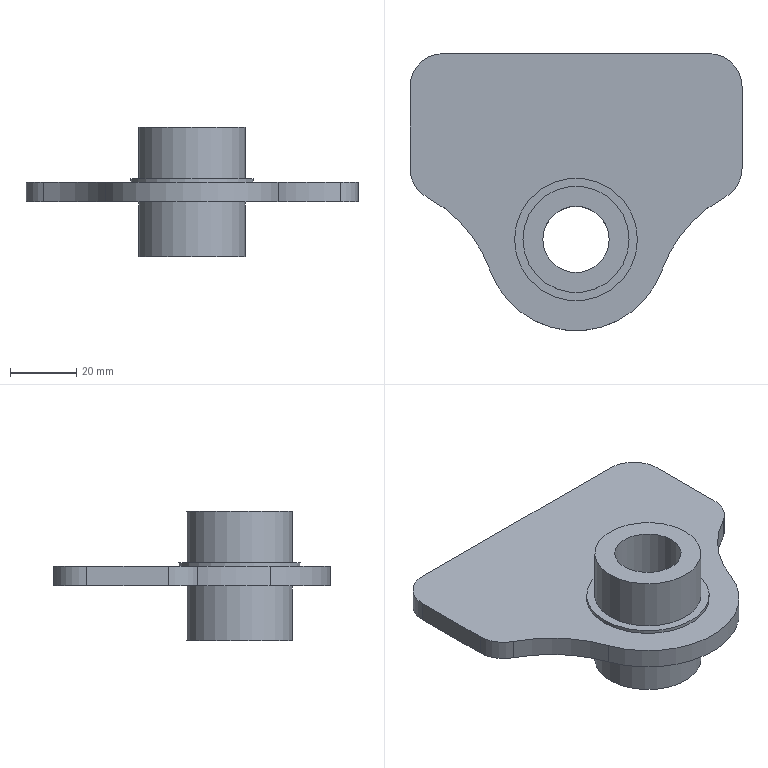NC program | NX | posted with a generic post | part box 100 x 83.5 x 39 mm
Lines 1 to 906 of 3591:
N10 G17 G21 G94 G90
(ADAPTIVE_MILLING , TOOL : D16-48-D16-100-3T-FINISH)
N12 T01 M6
N14 G53
N16 G17 G0 G90 X-29.129 Y-11.877 S3000 M3
N18 G43 Z30. H1
N20 Z3.15
N22 G94 G1 X-28.979 Y-11.865 Z2.213 F2000.
N24 X-28.829 Y-11.854 Z1.842
N26 X-28.68 Y-11.842 Z1.57
N28 X-28.53 Y-11.831 Z1.35
N30 X-28.381 Y-11.819 Z1.166
N32 X-28.231 Y-11.808 Z1.008
N34 X-28.082 Y-11.796 Z0.87
N36 X-27.932 Y-11.785 Z0.75
N38 X-27.783 Y-11.773 Z0.645
N40 X-27.633 Y-11.762 Z0.552
N42 X-27.483 Y-11.75 Z0.471
N44 X-27.334 Y-11.739 Z0.4
N46 X-27.184 Y-11.727 Z0.34
N48 X-27.035 Y-11.716 Z0.288
N50 X-26.885 Y-11.704 Z0.245
N52 X-26.736 Y-11.693 Z0.211
N54 X-26.586 Y-11.681 Z0.184
N56 X-26.436 Y-11.67 Z0.165
N58 X-26.287 Y-11.658 Z0.154
N60 X-26.137 Y-11.647 Z0.15
N62 X-24.02 Y-11.484
N64 G3 X-22.555 Y-9.578 R1.616
N66 G1 X-23.473 Y-5.647
N68 G2 X-22.056 Y9.568 R25.074
N70 X-20.662 Y-12.268 R-24.039
N72 X-23.288 Y-4.358 R24.506
N74 X-17.653 Y15.653 R24.1
N76 X-19.314 Y-13.525 R-23.593
N78 X-23.013 Y-3.231 R23.544
N80 X-13.785 Y18.59 R23.495
N82 X-17.92 Y-14.622 R-23.141
N84 X-22.633 Y-2.662 R22.849
N86 X-11.014 Y19.837 R22.99
N88 X-16.545 Y-15.504 R-22.686
N90 X-22.228 Y-2.182 R22.315
N92 X-8.532 Y20.527 R22.498
N94 X-15.335 Y-16.071 R-22.227
N96 X-21.826 Y-1.358 R21.88
N98 X-5.19 Y21.138 R21.988
N100 X-14.251 Y-16.427 R-21.762
N102 X-21.39 Y-0.363 R21.453
N104 X-1.126 Y21.266 R21.473
N106 X-12.994 Y-16.848 R-21.29
N108 X-20.917 Y0.217 R20.985
N110 X1.005 Y20.795 R20.982
N112 X-12.004 Y-16.984 R-20.813
N114 X-20.383 Y1.367 R20.542
N116 X4.974 Y19.719 R20.469
N118 X-11.011 Y-17.069 R-20.328
N120 X-19.791 Y2.388 R20.075
N122 X7.915 Y18.2 R19.96
N124 X-10.001 Y-17.112 R-19.835
N126 X-19.13 Y3.418 R19.594
N128 X10.367 Y16.335 R19.447
N130 X-9.145 Y-17.018 R19.333
N132 X-18.337 Y4.66 R19.106
N134 X12.992 Y13.643 R18.923
N136 X-8.398 Y-16.83 R18.82
N138 X-16.984 Y7.044 R18.615
N140 X17.291 Y6.061 R18.375
N142 X-8.2 Y-16.341 R18.285
N144 X-13.274 Y11.907 R18.121
N146 X-17.828 Y-0.094 R-17.828
N148 G1 X-17.825 Y0.056 Z0.154
N150 X-17.823 Y0.206 Z0.165
N152 X-17.821 Y0.356 Z0.184
N154 X-17.818 Y0.506 Z0.211
N156 X-17.816 Y0.656 Z0.245
N158 X-17.813 Y0.806 Z0.288
N160 X-17.811 Y0.956 Z0.34
N162 X-17.809 Y1.106 Z0.4
N164 X-17.806 Y1.256 Z0.471
N166 X-17.804 Y1.406 Z0.552
N168 X-17.802 Y1.556 Z0.645
N170 X-17.799 Y1.706 Z0.75
N172 X-17.797 Y1.856 Z0.87
N174 X-17.795 Y2.006 Z1.008
N176 X-17.792 Y2.156 Z1.166
N178 X-17.79 Y2.306 Z1.35
N180 X-17.788 Y2.456 Z1.57
N182 X-17.785 Y2.606 Z1.842
N184 X-17.783 Y2.756 Z2.213
N186 X-17.78 Y2.906 Z3.15
N188 G0 Z30.
(PLANAR_MILL_1_COPY , TOOL : D16-48-D16-100-3T-FINISH)
N190 X-13.655 Y22.716
N192 Z-12.4
N194 G1 X-12.158 Y23.58 Z-12.409 F1000.
N196 X-8.916 Y24.987 Z-12.428
N198 X-5.517 Y25.95 Z-12.446
N200 X-2.019 Y26.453 Z-12.465
N202 X1.514 Y26.487 Z-12.483
N204 X5.02 Y26.051 Z-12.502
N206 X8.438 Y25.152 Z-12.52
N208 X11.706 Y23.808 Z-12.539
N210 X14.766 Y22.041 Z-12.557
N212 X17.564 Y19.884 Z-12.576
N214 X20.05 Y17.373 Z-12.594
N216 X22.181 Y14.555 Z-12.613
N218 X23.919 Y11.478 Z-12.631
N220 X25.232 Y8.197 Z-12.65
N222 X26.097 Y4.772 Z-12.668
N224 X26.5 Y1.261 Z-12.687
N226 Y-1.261 Z-12.7
N228 X26.093 Y-4.794 Z-12.718
N230 X25.218 Y-8.241 Z-12.737
N232 X23.889 Y-11.54 Z-12.756
N234 X22.131 Y-14.631 Z-12.774
N236 X19.975 Y-17.46 Z-12.793
N238 X17.46 Y-19.975 Z-12.812
N240 X14.631 Y-22.131 Z-12.83
N242 X11.54 Y-23.889 Z-12.849
N244 X8.241 Y-25.218 Z-12.867
N246 X4.794 Y-26.093 Z-12.886
N248 X1.261 Y-26.5 Z-12.905
N250 X-1.261 Z-12.918
N252 X-4.087 Y-26.213 Z-12.933
N254 X-6.866 Y-25.626 Z-12.948
N256 X-9.567 Y-24.745 Z-12.962
N258 X-12.158 Y-23.58 Z-12.977
N260 X-14.342 Y-22.319 Z-12.991
N262 X-17.181 Y-20.215 Z-13.009
N264 X-19.715 Y-17.753 Z-13.028
N266 X-21.899 Y-14.975 Z-13.046
N268 X-23.695 Y-11.932 Z-13.065
N270 X-25.071 Y-8.677 Z-13.083
N272 X-26.002 Y-5.269 Z-13.102
N274 X-26.471 Y-1.767 Z-13.12
N276 Y1.767 Z-13.139
N278 X-26.002 Y5.269 Z-13.157
N280 X-25.071 Y8.677 Z-13.176
N282 X-23.695 Y11.932 Z-13.194
N284 X-21.899 Y14.975 Z-13.213
N286 X-19.715 Y17.753 Z-13.231
N288 X-17.181 Y20.215 Z-13.25
N290 X-14.342 Y22.319 Z-13.268
N292 X-12.158 Y23.58 Z-13.281
N294 X-8.916 Y24.987 Z-13.3
N296 X-5.517 Y25.95 Z-13.318
N298 X-2.019 Y26.453 Z-13.337
N300 X1.514 Y26.487 Z-13.355
N302 X5.02 Y26.051 Z-13.374
N304 X8.438 Y25.152 Z-13.392
N306 X11.706 Y23.808 Z-13.411
N308 X14.766 Y22.041 Z-13.429
N310 X17.564 Y19.884 Z-13.448
N312 X20.05 Y17.373 Z-13.466
N314 X22.181 Y14.555 Z-13.485
N316 X23.919 Y11.478 Z-13.503
N318 X25.232 Y8.197 Z-13.522
N320 X26.097 Y4.772 Z-13.54
N322 X26.5 Y1.261 Z-13.559
N324 Y-1.261 Z-13.572
N326 X26.093 Y-4.794 Z-13.591
N328 X25.218 Y-8.241 Z-13.609
N330 X23.889 Y-11.54 Z-13.628
N332 X22.131 Y-14.631 Z-13.646
N334 X19.975 Y-17.46 Z-13.665
N336 X17.46 Y-19.975 Z-13.684
N338 X14.631 Y-22.131 Z-13.702
N340 X11.54 Y-23.889 Z-13.721
N342 X8.241 Y-25.218 Z-13.74
N344 X4.794 Y-26.093 Z-13.758
N346 X1.261 Y-26.5 Z-13.777
N348 X-1.261 Z-13.79
N350 X-4.087 Y-26.213 Z-13.805
N352 X-6.866 Y-25.626 Z-13.82
N354 X-9.567 Y-24.745 Z-13.835
N356 X-12.158 Y-23.58 Z-13.85
N358 X-14.342 Y-22.319 Z-13.863
N360 X-17.181 Y-20.215 Z-13.881
N362 X-19.715 Y-17.753 Z-13.9
N364 X-21.899 Y-14.975 Z-13.918
N366 X-23.695 Y-11.932 Z-13.937
N368 X-25.071 Y-8.677 Z-13.955
N370 X-26.002 Y-5.269 Z-13.974
N372 X-26.471 Y-1.767 Z-13.992
N374 Y1.767 Z-14.011
N376 X-26.002 Y5.269 Z-14.029
N378 X-25.071 Y8.677 Z-14.048
N380 X-23.695 Y11.932 Z-14.066
N382 X-21.899 Y14.975 Z-14.085
N384 X-19.715 Y17.753 Z-14.103
N386 X-17.181 Y20.215 Z-14.122
N388 X-14.342 Y22.319 Z-14.14
N390 X-12.158 Y23.58 Z-14.153
N392 X-8.916 Y24.987 Z-14.172
N394 X-5.517 Y25.95 Z-14.19
N396 X-2.019 Y26.453 Z-14.209
N398 X1.514 Y26.487 Z-14.227
N400 X5.02 Y26.051 Z-14.246
N402 X8.438 Y25.152 Z-14.264
N404 X11.706 Y23.808 Z-14.283
N406 X14.766 Y22.041 Z-14.301
N408 X17.564 Y19.884 Z-14.32
N410 X20.05 Y17.373 Z-14.338
N412 X22.181 Y14.555 Z-14.357
N414 X23.919 Y11.478 Z-14.375
N416 X25.232 Y8.197 Z-14.394
N418 X26.097 Y4.772 Z-14.412
N420 X26.5 Y1.261 Z-14.431
N422 Y-1.261 Z-14.444
N424 X26.093 Y-4.794 Z-14.463
N426 X25.218 Y-8.241 Z-14.481
N428 X23.889 Y-11.54 Z-14.5
N430 X22.131 Y-14.631 Z-14.519
N432 X19.975 Y-17.46 Z-14.537
N434 X17.46 Y-19.975 Z-14.556
N436 X14.631 Y-22.131 Z-14.575
N438 X11.54 Y-23.889 Z-14.593
N440 X8.241 Y-25.218 Z-14.612
N442 X4.794 Y-26.093 Z-14.63
N444 X1.261 Y-26.5 Z-14.649
N446 X-1.261 Z-14.662
N448 X-4.087 Y-26.213 Z-14.677
N450 X-6.866 Y-25.626 Z-14.692
N452 X-9.567 Y-24.745 Z-14.707
N454 X-12.158 Y-23.58 Z-14.722
N456 X-14.342 Y-22.319 Z-14.735
N458 X-17.181 Y-20.215 Z-14.753
N460 X-19.715 Y-17.753 Z-14.772
N462 X-21.899 Y-14.975 Z-14.79
N464 X-23.695 Y-11.932 Z-14.809
N466 X-25.071 Y-8.677 Z-14.827
N468 X-26.002 Y-5.269 Z-14.846
N470 X-26.471 Y-1.767 Z-14.864
N472 Y1.767 Z-14.883
N474 X-26.002 Y5.269 Z-14.901
N476 X-25.071 Y8.677 Z-14.92
N478 X-23.695 Y11.932 Z-14.938
N480 X-21.899 Y14.975 Z-14.957
N482 X-19.715 Y17.753 Z-14.975
N484 X-17.181 Y20.215 Z-14.994
N486 X-14.342 Y22.319 Z-15.012
N488 X-12.158 Y23.58 Z-15.026
N490 X-8.916 Y24.987 Z-15.044
N492 X-5.517 Y25.95 Z-15.063
N494 X-2.019 Y26.453 Z-15.081
N496 X1.514 Y26.487 Z-15.1
N498 X5.02 Y26.051 Z-15.118
N500 X8.438 Y25.152 Z-15.137
N502 X11.706 Y23.808 Z-15.155
N504 X14.766 Y22.041 Z-15.174
N506 X17.564 Y19.884 Z-15.192
N508 X20.05 Y17.373 Z-15.211
N510 X22.181 Y14.555 Z-15.229
N512 X23.919 Y11.478 Z-15.248
N514 X25.232 Y8.197 Z-15.266
N516 X26.097 Y4.772 Z-15.285
N518 X26.5 Y1.261 Z-15.303
N520 Y-1.261 Z-15.316
N522 X26.093 Y-4.794 Z-15.335
N524 X25.218 Y-8.241 Z-15.354
N526 X23.889 Y-11.54 Z-15.372
N528 X22.131 Y-14.631 Z-15.391
N530 X19.975 Y-17.46 Z-15.409
N532 X17.46 Y-19.975 Z-15.428
N534 X14.631 Y-22.131 Z-15.447
N536 X11.54 Y-23.889 Z-15.465
N538 X8.241 Y-25.218 Z-15.484
N540 X4.794 Y-26.093 Z-15.503
N542 X1.261 Y-26.5 Z-15.521
N544 X-1.261 Z-15.534
N546 X-4.087 Y-26.213 Z-15.549
N548 X-6.866 Y-25.626 Z-15.564
N550 X-9.567 Y-24.745 Z-15.579
N552 X-12.158 Y-23.58 Z-15.594
N554 X-14.342 Y-22.319 Z-15.607
N556 X-17.181 Y-20.215 Z-15.626
N558 X-19.715 Y-17.753 Z-15.644
N560 X-21.899 Y-14.975 Z-15.663
N562 X-23.695 Y-11.932 Z-15.681
N564 X-25.071 Y-8.677 Z-15.7
N566 X-26.002 Y-5.269 Z-15.718
N568 X-26.471 Y-1.767 Z-15.737
N570 Y1.767 Z-15.755
N572 X-26.002 Y5.269 Z-15.774
N574 X-25.071 Y8.677 Z-15.792
N576 X-23.695 Y11.932 Z-15.811
N578 X-21.899 Y14.975 Z-15.829
N580 X-19.715 Y17.753 Z-15.848
N582 X-17.181 Y20.215 Z-15.866
N584 X-14.342 Y22.319 Z-15.885
N586 X-12.158 Y23.58 Z-15.898
N588 X-8.916 Y24.987 Z-15.916
N590 X-5.517 Y25.95 Z-15.935
N592 X-2.019 Y26.453 Z-15.953
N594 X1.514 Y26.487 Z-15.972
N596 X5.02 Y26.051 Z-15.99
N598 X8.438 Y25.152 Z-16.009
N600 X11.706 Y23.808 Z-16.027
N602 X14.766 Y22.041 Z-16.046
N604 X17.564 Y19.884 Z-16.064
N606 X20.05 Y17.373 Z-16.083
N608 X22.181 Y14.555 Z-16.101
N610 X23.919 Y11.478 Z-16.12
N612 X25.232 Y8.197 Z-16.138
N614 X26.097 Y4.772 Z-16.157
N616 X26.5 Y1.261 Z-16.175
N618 Y-1.261 Z-16.189
N620 X26.093 Y-4.794 Z-16.207
N622 X25.218 Y-8.241 Z-16.226
N624 X23.889 Y-11.54 Z-16.244
N626 X22.131 Y-14.631 Z-16.263
N628 X19.975 Y-17.46 Z-16.282
N630 X17.46 Y-19.975 Z-16.3
N632 X14.631 Y-22.131 Z-16.319
N634 X11.54 Y-23.889 Z-16.338
N636 X8.241 Y-25.218 Z-16.356
N638 X4.794 Y-26.093 Z-16.375
N640 X1.261 Y-26.5 Z-16.393
N642 X0. Z-16.4
N644 G2 X-26.5 Y0. R26.5
N646 X0. Y-26.5 R-26.5
N648 G1 Z-12.4
N650 G0 Z30.
(PLANAR_MILL , TOOL : D16-48-D16-100-3T-FINISH)
N652 X-25.515 Y-5.
N654 Z3.
N656 G1 Z0.
N658 X-21.
N660 G3 X-16. Y0. R5.
N662 G2 X0. Y16. R16.
N664 X-16. Y0. R-16.
N666 G3 X-21. Y5. R5.
N668 G1 X-25.515
N670 Z3.
N672 G0 Z30.
(FLOOR_WALL , TOOL : D16-48-D16-100-3T-FINISH)
N674 X-4. Y67.
N676 Z-11.5
N678 G1 Z-14.5
N680 Y56.
N682 G3 X0. Y52. R4.
N684 G1 X40.
N686 G2 X46. Y46. R6.
N688 G1 Y21.463
N690 G2 X42.83 Y16.173 R6.
N692 G3 X26.481 Y1.011 R44.
N694 X-26.481 Y1.011 R26.5
N696 X-42.832 Y16.174 R44.
N698 G2 X-46. Y21.463 R6.
N700 G1 Y46.
N702 G2 X-40. Y52. R6.
N704 G1 X0.
N706 Y40.
N708 X34.
N710 Y24.921
N712 G3 X30.959 Y22.887 R56.
N714 X-30.959 Y22.887 R38.5
N716 X-34. Y24.921 R56.
N718 G1 Y40.
N720 X0.
N722 X1.
N724 G3 X5. Y44. R4.
N726 G1 Z-11.5
N728 G0 Z30.
N730 X-4. Y67.
N732 Z-12.5
N734 G1 Z-15.5
N736 Y56.
N738 G3 X0. Y52. R4.
N740 G1 X40.
N742 G2 X46. Y46. R6.
N744 G1 Y21.463
N746 G2 X42.83 Y16.173 R6.
N748 G3 X26.481 Y1.011 R44.
N750 X-26.481 Y1.011 R26.5
N752 X-42.832 Y16.174 R44.
N754 G2 X-46. Y21.463 R6.
N756 G1 Y46.
N758 G2 X-40. Y52. R6.
N760 G1 X0.
N762 Y40.
N764 X34.
N766 Y24.921
N768 G3 X30.959 Y22.887 R56.
N770 X-30.959 Y22.887 R38.5
N772 X-34. Y24.921 R56.
N774 G1 Y40.
N776 X0.
N778 X1.
N780 G3 X5. Y44. R4.
N782 G1 Z-12.5
N784 G0 Z30.
N786 X-4. Y67.
N788 Z-13.5
N790 G1 Z-16.5
N792 Y56.
N794 G3 X0. Y52. R4.
N796 G1 X40.
N798 G2 X46. Y46. R6.
N800 G1 Y21.463
N802 G2 X42.83 Y16.173 R6.
N804 G3 X26.481 Y1.011 R44.
N806 X-26.481 Y1.011 R26.5
N808 X-42.832 Y16.174 R44.
N810 G2 X-46. Y21.463 R6.
N812 G1 Y46.
N814 G2 X-40. Y52. R6.
N816 G1 X0.
N818 Y40.
N820 X34.
N822 Y24.921
N824 G3 X30.959 Y22.887 R56.
N826 X-30.959 Y22.887 R38.5
N828 X-34. Y24.921 R56.
N830 G1 Y40.
N832 X0.
N834 X1.
N836 G3 X5. Y44. R4.
N838 G1 Z-13.5
N840 G0 Z30.
(PLANAR_MILL_1 , TOOL : D16-48-D16-100-3T-FINISH)
N842 Y-36.156
N844 Z-14.5
N846 G1 Z-16.5
N848 Y-31.5
N850 G3 X0. Y-26.5 R5.
N852 G2 X-26.5 Y0. R26.5
N854 X0. Y-26.5 R-26.5
N856 G3 X-5. Y-31.5 R5.
N858 G1 Y-36.156
N860 Z-14.5
N862 G0 Z30.
(PLANAR_MILL_4 , TOOL : D16-48-D16-100-3T-FINISH)
N864 X-0.159 Y1.88
N866 Z1.
N868 G1 X-0.656 Y1.815 Z0.991
N870 X-1.244 Y1.476 Z0.979
N872 X-1.671 Y0.965 Z0.968
N874 X-1.9 Y0.339 Z0.956
N876 Y-0.339 Z0.944
N878 X-1.671 Y-0.965 Z0.933
N880 X-1.244 Y-1.476 Z0.921
N882 X-0.656 Y-1.815 Z0.909
N884 X0.17 Y-1.922 Z0.895
N886 X0.965 Y-1.671 Z0.88
N888 X1.58 Y-1.109 Z0.866
N890 X1.9 Y-0.339 Z0.851
N892 Y0.339 Z0.839
N894 X1.58 Y1.109 Z0.825
N896 X0.965 Y1.671 Z0.81
N898 X0.17 Y1.922 Z0.796
N900 X-0.656 Y1.815 Z0.781
N902 X-1.244 Y1.476 Z0.769
N904 X-1.671 Y0.965 Z0.758
N906 X-1.9 Y0.339 Z0.746
N908 Y-0.339 Z0.734
N910 X-1.671 Y-0.965 Z0.722
N912 X-1.244 Y-1.476 Z0.711
N914 X-0.656 Y-1.815 Z0.699
N916 X0.17 Y-1.922 Z0.684
N918 X0.965 Y-1.671 Z0.67
N920 X1.58 Y-1.109 Z0.655
N922 X1.9 Y-0.339 Z0.641
N924 Y0.339 Z0.629
N926 X1.58 Y1.109 Z0.614
N928 X0.965 Y1.671 Z0.6
N930 X0.17 Y1.922 Z0.585
N932 X-0.656 Y1.815 Z0.571
N934 X-1.244 Y1.476 Z0.559
N936 X-1.671 Y0.965 Z0.547
N938 X-1.9 Y0.339 Z0.536
N940 Y-0.339 Z0.524
N942 X-1.671 Y-0.965 Z0.512
N944 X-1.244 Y-1.476 Z0.501
N946 X-0.656 Y-1.815 Z0.489
N948 X0.17 Y-1.922 Z0.474
N950 X0.965 Y-1.671 Z0.46
N952 X1.58 Y-1.109 Z0.445
N954 X1.9 Y-0.339 Z0.43
N956 Y0.339 Z0.419
N958 X1.58 Y1.109 Z0.404
N960 X0.965 Y1.671 Z0.39
N962 X0.17 Y1.922 Z0.375
N964 X-0.656 Y1.815 Z0.36
N966 X-1.244 Y1.476 Z0.349
N968 X-1.671 Y0.965 Z0.337
N970 X-1.9 Y0.339 Z0.325
N972 Y-0.339 Z0.314
N974 X-1.671 Y-0.965 Z0.302
N976 X-1.244 Y-1.476 Z0.29
N978 X-0.656 Y-1.815 Z0.278
N980 X0.17 Y-1.922 Z0.264
N982 X0.965 Y-1.671 Z0.249
N984 X1.58 Y-1.109 Z0.235
N986 X1.9 Y-0.339 Z0.22
N988 Y0.339 Z0.208
N990 X1.58 Y1.109 Z0.194
N992 X0.965 Y1.671 Z0.179
N994 X0.17 Y1.922 Z0.165
N996 X-0.656 Y1.815 Z0.15
N998 X-1.244 Y1.476 Z0.138
N1000 X-1.671 Y0.965 Z0.127
N1002 X-1.9 Y0.339 Z0.115
N1004 Y-0.339 Z0.103
N1006 X-1.671 Y-0.965 Z0.092
N1008 X-1.244 Y-1.476 Z0.08
N1010 X-0.656 Y-1.815 Z0.068
N1012 X0.17 Y-1.922 Z0.054
N1014 X0.965 Y-1.671 Z0.039
N1016 X1.58 Y-1.109 Z0.025
N1018 X1.9 Y-0.339 Z0.01
N1020 Y0.339 Z-0.002
N1022 X1.58 Y1.109 Z-0.016
N1024 X0.965 Y1.671 Z-0.031
N1026 X0.17 Y1.922 Z-0.046
N1028 X-0.656 Y1.815 Z-0.06
N1030 X-1.244 Y1.476 Z-0.072
N1032 X-1.671 Y0.965 Z-0.084
N1034 X-1.9 Y0.339 Z-0.095
N1036 Y-0.339 Z-0.107
N1038 X-1.671 Y-0.965 Z-0.119
N1040 X-1.244 Y-1.476 Z-0.13
N1042 X-0.656 Y-1.815 Z-0.142
N1044 X0.17 Y-1.922 Z-0.157
N1046 X0.965 Y-1.671 Z-0.171
N1048 X1.58 Y-1.109 Z-0.186
N1050 X1.9 Y-0.339 Z-0.2
N1052 Y0.339 Z-0.212
N1054 X1.58 Y1.109 Z-0.227
N1056 X0.965 Y1.671 Z-0.241
N1058 X0.17 Y1.922 Z-0.256
N1060 X-0.656 Y1.815 Z-0.27
N1062 X-1.244 Y1.476 Z-0.282
N1064 X-1.671 Y0.965 Z-0.294
N1066 X-1.9 Y0.339 Z-0.305
N1068 Y-0.339 Z-0.317
N1070 X-1.671 Y-0.965 Z-0.329
N1072 X-1.244 Y-1.476 Z-0.341
N1074 X-0.656 Y-1.815 Z-0.352
N1076 X0.17 Y-1.922 Z-0.367
N1078 X0.965 Y-1.671 Z-0.381
N1080 X1.58 Y-1.109 Z-0.396
N1082 X1.9 Y-0.339 Z-0.411
N1084 Y0.339 Z-0.422
N1086 X1.58 Y1.109 Z-0.437
N1088 X0.965 Y1.671 Z-0.452
N1090 X0.17 Y1.922 Z-0.466
N1092 X-0.656 Y1.815 Z-0.481
N1094 X-1.244 Y1.476 Z-0.492
N1096 X-1.671 Y0.965 Z-0.504
N1098 X-1.9 Y0.339 Z-0.516
N1100 Y-0.339 Z-0.528
N1102 X-1.671 Y-0.965 Z-0.539
N1104 X-1.244 Y-1.476 Z-0.551
N1106 X-0.656 Y-1.815 Z-0.563
N1108 X0.17 Y-1.922 Z-0.577
N1110 X0.965 Y-1.671 Z-0.592
N1112 X1.58 Y-1.109 Z-0.606
N1114 X1.9 Y-0.339 Z-0.621
N1116 Y0.339 Z-0.633
N1118 X1.58 Y1.109 Z-0.647
N1120 X0.965 Y1.671 Z-0.662
N1122 X0.17 Y1.922 Z-0.676
N1124 X-0.656 Y1.815 Z-0.691
N1126 X-1.244 Y1.476 Z-0.703
N1128 X-1.671 Y0.965 Z-0.714
N1130 X-1.9 Y0.339 Z-0.726
N1132 Y-0.339 Z-0.738
N1134 X-1.671 Y-0.965 Z-0.749
N1136 X-1.244 Y-1.476 Z-0.761
N1138 X-0.656 Y-1.815 Z-0.773
N1140 X0.17 Y-1.922 Z-0.787
N1142 X0.965 Y-1.671 Z-0.802
N1144 X1.58 Y-1.109 Z-0.817
N1146 X1.9 Y-0.339 Z-0.831
N1148 Y0.339 Z-0.843
N1150 X1.58 Y1.109 Z-0.857
N1152 X0.965 Y1.671 Z-0.872
N1154 X0.17 Y1.922 Z-0.887
N1156 X-0.656 Y1.815 Z-0.901
N1158 X-1.244 Y1.476 Z-0.913
N1160 X-1.671 Y0.965 Z-0.925
N1162 X-1.9 Y0.339 Z-0.936
N1164 Y-0.339 Z-0.948
N1166 X-1.671 Y-0.965 Z-0.96
N1168 X-1.244 Y-1.476 Z-0.971
N1170 X-0.656 Y-1.815 Z-0.983
N1172 X0.17 Y-1.922 Z-0.998
N1174 X0.965 Y-1.671 Z-1.012
N1176 X1.58 Y-1.109 Z-1.027
N1178 X1.9 Y-0.339 Z-1.041
N1180 Y0.339 Z-1.053
N1182 X1.58 Y1.109 Z-1.068
N1184 X0.965 Y1.671 Z-1.082
N1186 X0.17 Y1.922 Z-1.097
N1188 X-0.656 Y1.815 Z-1.111
N1190 X-1.244 Y1.476 Z-1.123
N1192 X-1.671 Y0.965 Z-1.135
N1194 X-1.9 Y0.339 Z-1.147
N1196 Y-0.339 Z-1.158
N1198 X-1.671 Y-0.965 Z-1.17
N1200 X-1.244 Y-1.476 Z-1.182
N1202 X-0.656 Y-1.815 Z-1.193
N1204 X0.17 Y-1.922 Z-1.208
N1206 X0.965 Y-1.671 Z-1.223
N1208 X1.58 Y-1.109 Z-1.237
N1210 X1.9 Y-0.339 Z-1.252
N1212 Y0.339 Z-1.263
N1214 X1.58 Y1.109 Z-1.278
N1216 X0.965 Y1.671 Z-1.293
N1218 X0.17 Y1.922 Z-1.307
N1220 X-0.656 Y1.815 Z-1.322
N1222 X-1.244 Y1.476 Z-1.334
N1224 X-1.671 Y0.965 Z-1.345
N1226 X-1.9 Y0.339 Z-1.357
N1228 Y-0.339 Z-1.369
N1230 X-1.671 Y-0.965 Z-1.38
N1232 X-1.244 Y-1.476 Z-1.392
N1234 X-0.656 Y-1.815 Z-1.404
N1236 X0.17 Y-1.922 Z-1.418
N1238 X0.965 Y-1.671 Z-1.433
N1240 X1.58 Y-1.109 Z-1.447
N1242 X1.9 Y-0.339 Z-1.462
N1244 Y0.339 Z-1.474
N1246 X1.58 Y1.109 Z-1.488
N1248 X0.965 Y1.671 Z-1.503
N1250 X0.17 Y1.922 Z-1.517
N1252 X-0.656 Y1.815 Z-1.532
N1254 X-1.244 Y1.476 Z-1.544
N1256 X-1.671 Y0.965 Z-1.555
N1258 X-1.9 Y0.339 Z-1.567
N1260 Y-0.339 Z-1.579
N1262 X-1.671 Y-0.965 Z-1.59
N1264 X-1.244 Y-1.476 Z-1.602
N1266 X-0.656 Y-1.815 Z-1.614
N1268 X0.17 Y-1.922 Z-1.629
N1270 X0.965 Y-1.671 Z-1.643
N1272 X1.58 Y-1.109 Z-1.658
N1274 X1.9 Y-0.339 Z-1.672
N1276 Y0.339 Z-1.684
N1278 X1.58 Y1.109 Z-1.699
N1280 X0.965 Y1.671 Z-1.713
N1282 X0.17 Y1.922 Z-1.728
N1284 X-0.656 Y1.815 Z-1.742
N1286 X-1.244 Y1.476 Z-1.754
N1288 X-1.671 Y0.965 Z-1.766
N1290 X-1.9 Y0.339 Z-1.777
N1292 Y-0.339 Z-1.789
N1294 X-1.671 Y-0.965 Z-1.801
N1296 X-1.244 Y-1.476 Z-1.812
N1298 X-0.656 Y-1.815 Z-1.824
N1300 X0.17 Y-1.922 Z-1.839
N1302 X0.965 Y-1.671 Z-1.853
N1304 X1.58 Y-1.109 Z-1.868
N1306 X1.9 Y-0.339 Z-1.882
N1308 Y0.339 Z-1.894
N1310 X1.58 Y1.109 Z-1.909
N1312 X0.965 Y1.671 Z-1.923
N1314 X0.17 Y1.922 Z-1.938
N1316 X-0.656 Y1.815 Z-1.952
N1318 X-1.244 Y1.476 Z-1.964
N1320 X-1.671 Y0.965 Z-1.976
N1322 X-1.9 Y0.339 Z-1.988
N1324 Y-0.339 Z-1.999
N1326 X-1.671 Y-0.965 Z-2.011
N1328 X-1.244 Y-1.476 Z-2.023
N1330 X-0.656 Y-1.815 Z-2.034
N1332 X0.17 Y-1.922 Z-2.049
N1334 X0.965 Y-1.671 Z-2.064
N1336 X1.58 Y-1.109 Z-2.078
N1338 X1.9 Y-0.339 Z-2.093
N1340 Y0.339 Z-2.105
N1342 X1.58 Y1.109 Z-2.119
N1344 X0.965 Y1.671 Z-2.134
N1346 X0.17 Y1.922 Z-2.148
N1348 X-0.656 Y1.815 Z-2.163
N1350 X-1.244 Y1.476 Z-2.175
N1352 X-1.671 Y0.965 Z-2.186
N1354 X-1.9 Y0.339 Z-2.198
N1356 Y-0.339 Z-2.21
N1358 X-1.671 Y-0.965 Z-2.221
N1360 X-1.244 Y-1.476 Z-2.233
N1362 X-0.656 Y-1.815 Z-2.245
N1364 X0.17 Y-1.922 Z-2.259
N1366 X0.965 Y-1.671 Z-2.274
N1368 X1.58 Y-1.109 Z-2.288
N1370 X1.9 Y-0.339 Z-2.303
N1372 Y0.339 Z-2.315
N1374 X1.58 Y1.109 Z-2.329
N1376 X0.965 Y1.671 Z-2.344
N1378 X0.17 Y1.922 Z-2.358
N1380 X-0.656 Y1.815 Z-2.373
N1382 X-1.244 Y1.476 Z-2.385
N1384 X-1.671 Y0.965 Z-2.396
N1386 X-1.9 Y0.339 Z-2.408
N1388 Y-0.339 Z-2.42
N1390 X-1.671 Y-0.965 Z-2.432
N1392 X-1.244 Y-1.476 Z-2.443
N1394 X-0.656 Y-1.815 Z-2.455
N1396 X0.17 Y-1.922 Z-2.47
N1398 X0.965 Y-1.671 Z-2.484
N1400 X1.58 Y-1.109 Z-2.499
N1402 X1.9 Y-0.339 Z-2.513
N1404 Y0.339 Z-2.525
N1406 X1.58 Y1.109 Z-2.54
N1408 X0.965 Y1.671 Z-2.554
N1410 X0.17 Y1.922 Z-2.569
N1412 X-0.656 Y1.815 Z-2.583
N1414 X-1.244 Y1.476 Z-2.595
N1416 X-1.671 Y0.965 Z-2.607
N1418 X-1.9 Y0.339 Z-2.618
N1420 Y-0.339 Z-2.63
N1422 X-1.671 Y-0.965 Z-2.642
N1424 X-1.244 Y-1.476 Z-2.653
N1426 X-0.656 Y-1.815 Z-2.665
N1428 X0.17 Y-1.922 Z-2.68
N1430 X0.965 Y-1.671 Z-2.694
N1432 X1.58 Y-1.109 Z-2.709
N1434 X1.9 Y-0.339 Z-2.723
N1436 Y0.339 Z-2.735
N1438 X1.58 Y1.109 Z-2.75
N1440 X0.965 Y1.671 Z-2.764
N1442 X0.17 Y1.922 Z-2.779
N1444 X-0.656 Y1.815 Z-2.794
N1446 X-1.244 Y1.476 Z-2.805
N1448 X-1.671 Y0.965 Z-2.817
N1450 X-1.9 Y0.339 Z-2.829
N1452 Y-0.339 Z-2.84
N1454 X-1.671 Y-0.965 Z-2.852
N1456 X-1.244 Y-1.476 Z-2.864
N1458 X-0.656 Y-1.815 Z-2.876
N1460 X0.17 Y-1.922 Z-2.89
N1462 X0.965 Y-1.671 Z-2.905
N1464 X1.58 Y-1.109 Z-2.919
N1466 X1.9 Y-0.339 Z-2.934
N1468 Y0.339 Z-2.946
N1470 X1.58 Y1.109 Z-2.96
N1472 X0.965 Y1.671 Z-2.975
N1474 X0.17 Y1.922 Z-2.989
N1476 X-0.656 Y1.815 Z-3.004
N1478 X-1.244 Y1.476 Z-3.016
N1480 X-1.671 Y0.965 Z-3.027
N1482 X-1.9 Y0.339 Z-3.039
N1484 Y-0.339 Z-3.051
N1486 X-1.671 Y-0.965 Z-3.062
N1488 X-1.244 Y-1.476 Z-3.074
N1490 X-0.656 Y-1.815 Z-3.086
N1492 X0.17 Y-1.922 Z-3.1
N1494 X0.965 Y-1.671 Z-3.115
N1496 X1.58 Y-1.109 Z-3.129
N1498 X1.9 Y-0.339 Z-3.144
N1500 Y0.339 Z-3.156
N1502 X1.58 Y1.109 Z-3.17
N1504 X0.965 Y1.671 Z-3.185
N1506 X0.17 Y1.922 Z-3.199
N1508 X-0.656 Y1.815 Z-3.214
N1510 X-1.244 Y1.476 Z-3.226
N1512 X-1.671 Y0.965 Z-3.238
N1514 X-1.9 Y0.339 Z-3.249
N1516 Y-0.339 Z-3.261
N1518 X-1.671 Y-0.965 Z-3.273
N1520 X-1.244 Y-1.476 Z-3.284
N1522 X-0.656 Y-1.815 Z-3.296
N1524 X0.17 Y-1.922 Z-3.311
N1526 X0.965 Y-1.671 Z-3.325
N1528 X1.58 Y-1.109 Z-3.34
N1530 X1.9 Y-0.339 Z-3.354
N1532 Y0.339 Z-3.366
N1534 X1.58 Y1.109 Z-3.381
N1536 X0.965 Y1.671 Z-3.395
N1538 X0.17 Y1.922 Z-3.41
N1540 X-0.656 Y1.815 Z-3.424
N1542 X-1.244 Y1.476 Z-3.436
N1544 X-1.671 Y0.965 Z-3.448
N1546 X-1.9 Y0.339 Z-3.459
N1548 Y-0.339 Z-3.471
N1550 X-1.671 Y-0.965 Z-3.483
N1552 X-1.244 Y-1.476 Z-3.495
N1554 X-0.656 Y-1.815 Z-3.506
N1556 X0.17 Y-1.922 Z-3.521
N1558 X0.965 Y-1.671 Z-3.535
N1560 X1.58 Y-1.109 Z-3.55
N1562 X1.9 Y-0.339 Z-3.565
N1564 Y0.339 Z-3.576
N1566 X1.58 Y1.109 Z-3.591
N1568 X0.965 Y1.671 Z-3.605
N1570 X0.17 Y1.922 Z-3.62
N1572 X-0.656 Y1.815 Z-3.635
N1574 X-1.244 Y1.476 Z-3.646
N1576 X-1.671 Y0.965 Z-3.658
N1578 X-1.9 Y0.339 Z-3.67
N1580 Y-0.339 Z-3.682
N1582 X-1.671 Y-0.965 Z-3.693
N1584 X-1.244 Y-1.476 Z-3.705
N1586 X-0.656 Y-1.815 Z-3.717
N1588 X0.17 Y-1.922 Z-3.731
N1590 X0.965 Y-1.671 Z-3.746
N1592 X1.58 Y-1.109 Z-3.76
N1594 X1.9 Y-0.339 Z-3.775
N1596 Y0.339 Z-3.787
N1598 X1.58 Y1.109 Z-3.801
N1600 X0.965 Y1.671 Z-3.816
N1602 X0.17 Y1.922 Z-3.83
N1604 X-0.656 Y1.815 Z-3.845
N1606 X-1.244 Y1.476 Z-3.857
N1608 X-1.671 Y0.965 Z-3.868
N1610 X-1.9 Y0.339 Z-3.88
N1612 Y-0.339 Z-3.892
N1614 X-1.671 Y-0.965 Z-3.903
N1616 X-1.244 Y-1.476 Z-3.915
N1618 X-0.656 Y-1.815 Z-3.927
N1620 X0.17 Y-1.922 Z-3.941
N1622 X0.965 Y-1.671 Z-3.956
N1624 X1.58 Y-1.109 Z-3.971
N1626 X1.9 Y-0.339 Z-3.985
N1628 Y0.339 Z-3.997
N1630 X1.58 Y1.109 Z-4.011
N1632 X0.965 Y1.671 Z-4.026
N1634 X0.17 Y1.922 Z-4.041
N1636 X-0.656 Y1.815 Z-4.055
N1638 X-1.244 Y1.476 Z-4.067
N1640 X-1.671 Y0.965 Z-4.079
N1642 X-1.9 Y0.339 Z-4.09
N1644 Y-0.339 Z-4.102
N1646 X-1.671 Y-0.965 Z-4.114
N1648 X-1.244 Y-1.476 Z-4.125
N1650 X-0.656 Y-1.815 Z-4.137
N1652 X0.17 Y-1.922 Z-4.152
N1654 X0.965 Y-1.671 Z-4.166
N1656 X1.58 Y-1.109 Z-4.181
N1658 X1.9 Y-0.339 Z-4.195
N1660 Y0.339 Z-4.207
N1662 X1.58 Y1.109 Z-4.222
N1664 X0.965 Y1.671 Z-4.236
N1666 X0.17 Y1.922 Z-4.251
N1668 X-0.656 Y1.815 Z-4.265
N1670 X-1.244 Y1.476 Z-4.277
N1672 X-1.671 Y0.965 Z-4.289
N1674 X-1.9 Y0.339 Z-4.3
N1676 Y-0.339 Z-4.312
N1678 X-1.671 Y-0.965 Z-4.324
N1680 X-1.244 Y-1.476 Z-4.336
N1682 X-0.656 Y-1.815 Z-4.347
N1684 X0.17 Y-1.922 Z-4.362
N1686 X0.965 Y-1.671 Z-4.377
N1688 X1.58 Y-1.109 Z-4.391
N1690 X1.9 Y-0.339 Z-4.406
N1692 Y0.339 Z-4.417
N1694 X1.58 Y1.109 Z-4.432
N1696 X0.965 Y1.671 Z-4.447
N1698 X0.17 Y1.922 Z-4.461
N1700 X-0.656 Y1.815 Z-4.476
N1702 X-1.244 Y1.476 Z-4.487
N1704 X-1.671 Y0.965 Z-4.499
N1706 X-1.9 Y0.339 Z-4.511
N1708 Y-0.339 Z-4.523
N1710 X-1.671 Y-0.965 Z-4.534
N1712 X-1.244 Y-1.476 Z-4.546
N1714 X-0.656 Y-1.815 Z-4.558
N1716 X0.17 Y-1.922 Z-4.572
N1718 X0.965 Y-1.671 Z-4.587
N1720 X1.58 Y-1.109 Z-4.601
N1722 X1.9 Y-0.339 Z-4.616
N1724 Y0.339 Z-4.628
N1726 X1.58 Y1.109 Z-4.642
N1728 X0.965 Y1.671 Z-4.657
N1730 X0.17 Y1.922 Z-4.671
N1732 X-0.656 Y1.815 Z-4.686
N1734 X-1.244 Y1.476 Z-4.698
N1736 X-1.671 Y0.965 Z-4.709
N1738 X-1.9 Y0.339 Z-4.721
N1740 Y-0.339 Z-4.733
N1742 X-1.671 Y-0.965 Z-4.744
N1744 X-1.244 Y-1.476 Z-4.756
N1746 X-0.656 Y-1.815 Z-4.768
N1748 X0.17 Y-1.922 Z-4.782
N1750 X0.965 Y-1.671 Z-4.797
N1752 X1.58 Y-1.109 Z-4.812
N1754 X1.9 Y-0.339 Z-4.826
N1756 Y0.339 Z-4.838
N1758 X1.58 Y1.109 Z-4.853
N1760 X0.965 Y1.671 Z-4.867
N1762 X0.17 Y1.922 Z-4.882
N1764 X-0.656 Y1.815 Z-4.896
N1766 X-1.244 Y1.476 Z-4.908
N1768 X-1.671 Y0.965 Z-4.92
N1770 X-1.9 Y0.339 Z-4.931
N1772 Y-0.339 Z-4.943
N1774 X-1.671 Y-0.965 Z-4.955
N1776 X-1.244 Y-1.476 Z-4.966
N1778 X-0.656 Y-1.815 Z-4.978
N1780 X0.17 Y-1.922 Z-4.993